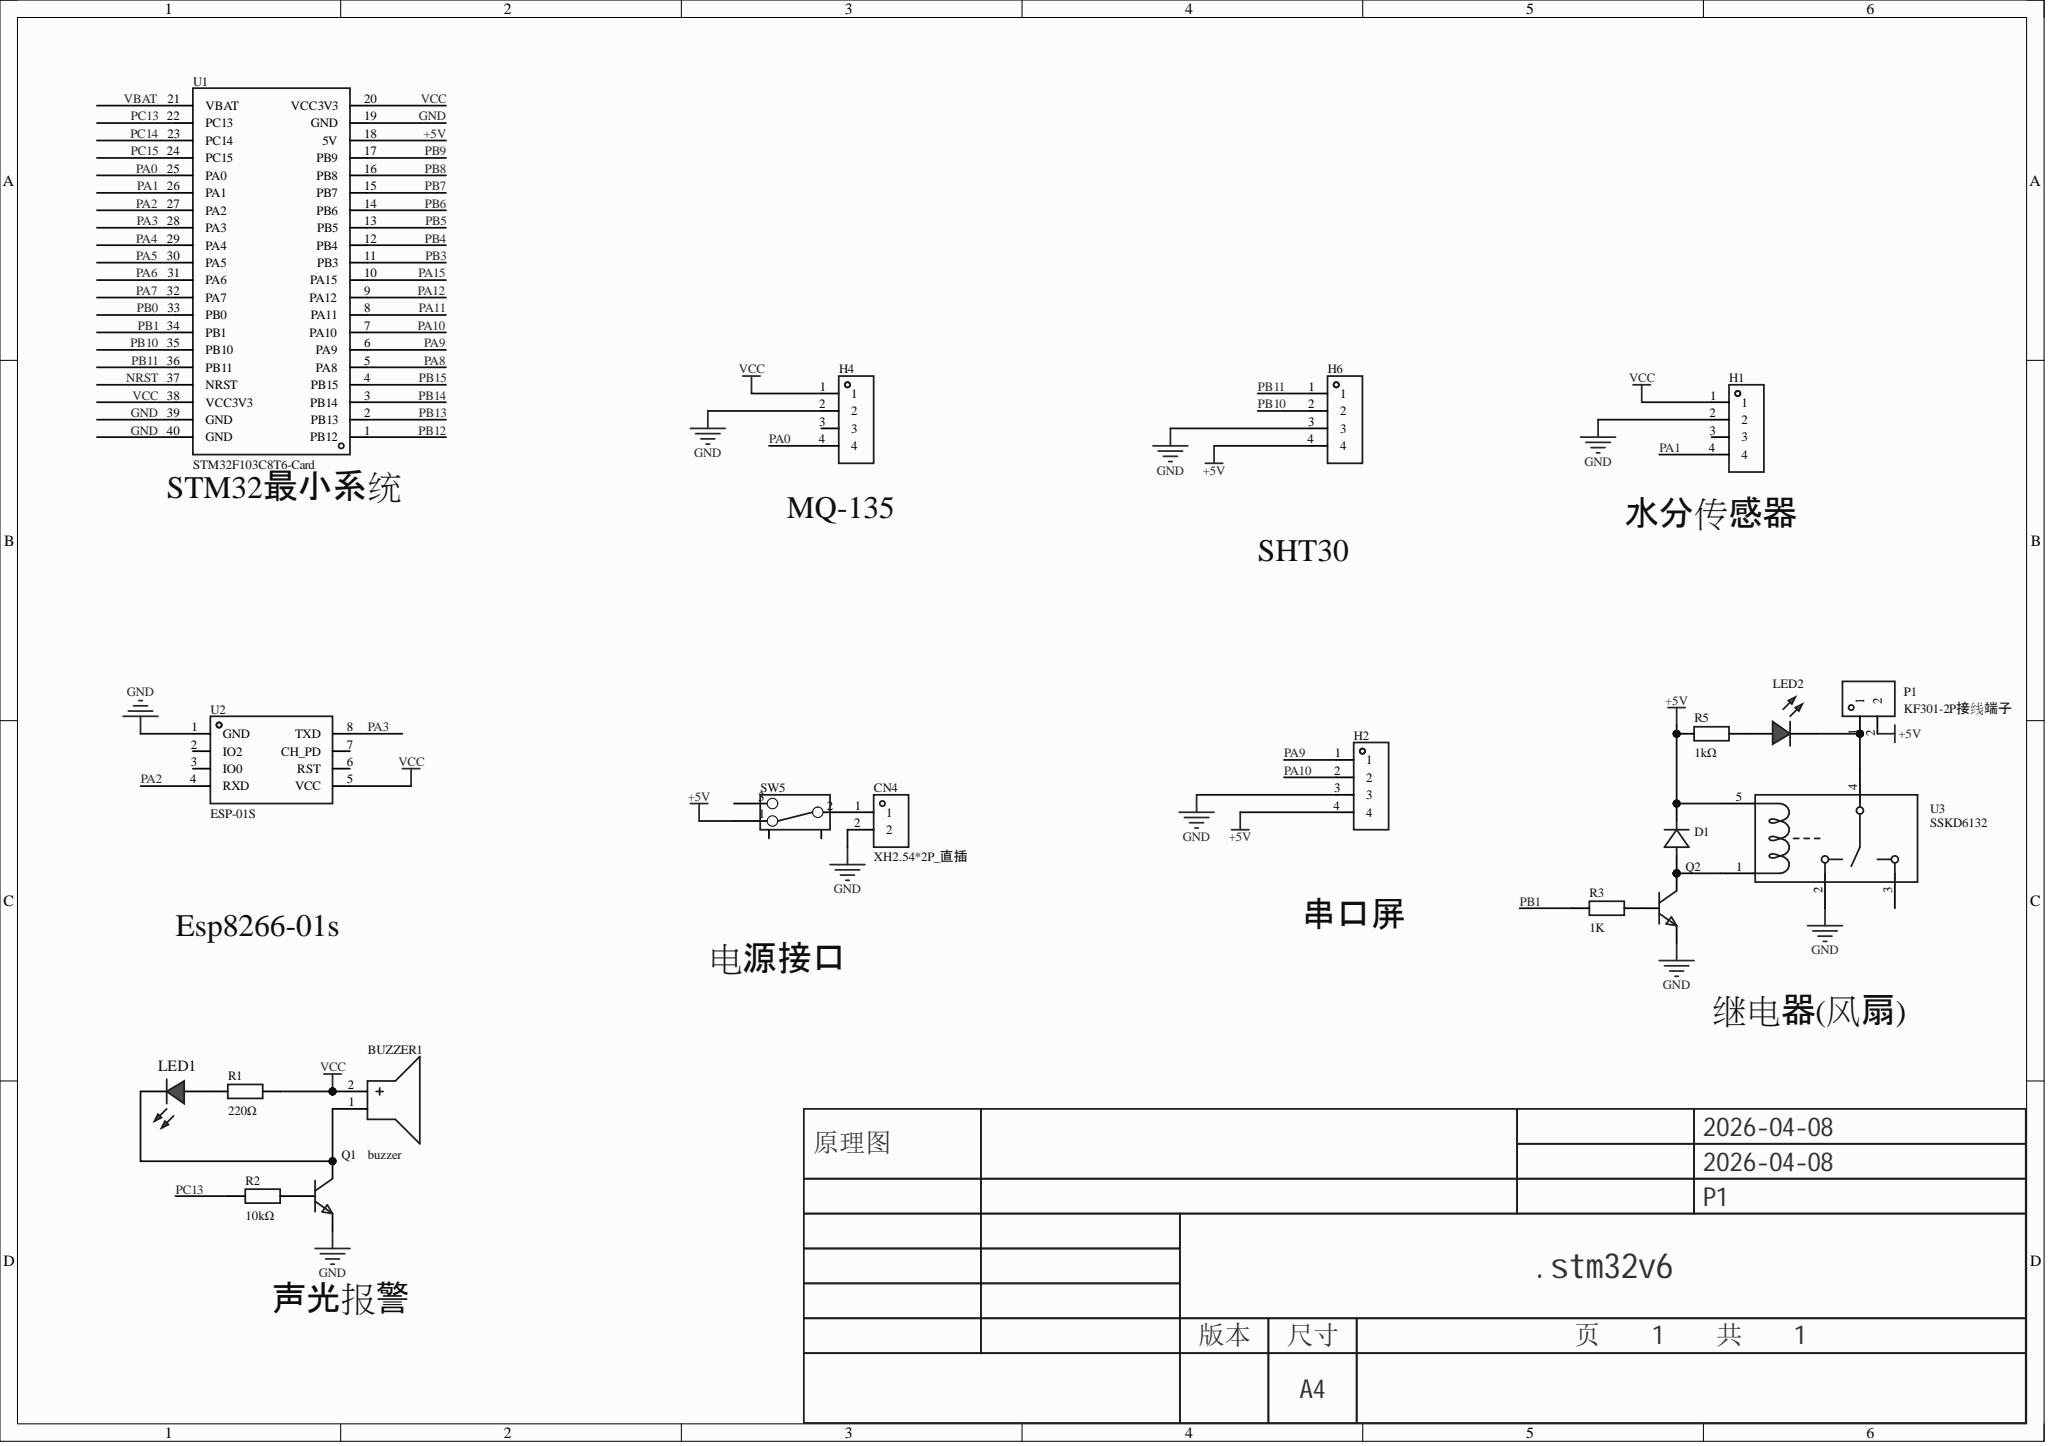Circuit board | Altium Designer | 20 parts | 21 nets
Bill of materials:
Comment,Description,Designator,Footprint,LibRef,Quantity
"buzzer","","BUZZER1","BUZ-TH_BD12.0-P6.00-D0.9-RD","buzzer","1"
"XH2.54*2P_直插","","CN4","CONN-TH_2P-P2.50-XH2.54-2P","XH2.54*2P_直插","1"
"","","D1","SMA_1N4007","D_1N4007","1"
"","","H1, H2, H4, H6","HDR-TH_4P-P2.54-V-F","HDR-F_2.54_1x4P","4"
"","","LED1","LED_0603","LED_0603-R","1"
"","","LED2","LED_TH-3mm","LED_TH-R_3mm","1"
"KF301-2P接线端子","","P1","CONN-TH_XY301V-A-5.0-2P","KF301-2P接线端子","1"
"","","Q1","S8050_TO_92","S8050_TO_NPN","1"
"","","Q2","S8050_SOT-23","S8050_SOT_NPN","1"
"220Ω","","R1","Res_1/8W","Res_AXIAL-1/8W","1"
"10kΩ","","R2","Res_1/8W","Res_AXIAL-1/8W","1"
"1K","","R3","R0603","Res_0603","1"
"1kΩ","","R5","Res_1/8W","Res_AXIAL-1/8W","1"
"","","SW5","拨动开关","拨动开关_正","1"
"STM32F103C8T6-Card","","U1","CONN-TH_L53.3-W22.9_STM32F103C8T6-CARD","STM32F103C8T6-Card","1"
"ESP-01S","","U2","WIFIM-TH_ESP-01S","ESP-01S_C111009","1"
"SSKD6132","","U3","RELAY-TH_G2R-1","SSKD6132","1"
Netlist (Protel format):
[
BUZZER1
BUZ-TH_BD12.0-P6.00-D0.9-RD
buzzer



]
[
CN4
CONN-TH_2P-P2.50-XH2.54-2P
XH2.54*2P_直插



]
[
D1
SMA_1N4007




]
[
H1
HDR-TH_4P-P2.54-V-F




]
[
H2
HDR-TH_4P-P2.54-V-F




]
[
H4
HDR-TH_4P-P2.54-V-F




]
[
H6
HDR-TH_4P-P2.54-V-F




]
[
LED1
LED_0603




]
[
LED2
LED_TH-3mm




]
[
P1
CONN-TH_XY301V-A-5.0-2P
KF301-2P接线端子



]
[
Q1
S8050_TO_92




]
[
Q2
S8050_SOT-23




]
[
R1
Res_1/8W
220Ω



]
[
R2
Res_1/8W
10kΩ



]
[
R3
R0603
1K



]
[
R5
Res_1/8W
1kΩ



]
[
SW5
拨动开关




]
[
U1
CONN-TH_L53.3-W22.9_STM32F103C8T6-CARD
STM32F103C8T6-Card



]
[
U2
WIFIM-TH_ESP-01S
ESP-01S



]
[
U3
RELAY-TH_G2R-1
SSKD6132



]
(
VCC
BUZZER1-2
H1-1
H4-1
R1-2
U1-20
U1-38
U2-5
)
(
PC13
R2-1
U1-22
)
(
PB11
H6-1
U1-36
)
(
PB10
H6-2
U1-35
)
(
PB1
R3-1
U1-34
)
(
PA10
H2-2
U1-7
)
(
PA9
H2-1
U1-6
)
(
PA3
U1-28
U2-8
)
(
PA2
U1-27
U2-4
)
(
PA1
H1-4
U1-26
)
(
PA0
H4-4
U1-25
)
(
NetQ2_1
Q2-1
R3-2
)
(
NetQ1_2
Q1-2
R2-2
)
(
NetLED2_2
LED2-2
P1-1
U3-4
)
(
NetLED2_1
LED2-1
R5-2
)
(
NetLED1_2
LED1-2
R1-1
)
(
NetD1_2
D1-2
Q2-3
U3-1
)
(
NetCN4_1
CN4-1
SW5-2
)
(
NetBUZZER1_1
BUZZER1-1
LED1-1
Q1-3
)
(
GND
CN4-2
H1-2
H2-3
H4-2
H6-3
Q1-1
Q2-2
U1-19
U1-39
U1-40
U2-1
U3-2
)
(
+5V
D1-1
H2-4
H6-4
P1-2
R5-1
SW5-1
U1-18
U3-5
)